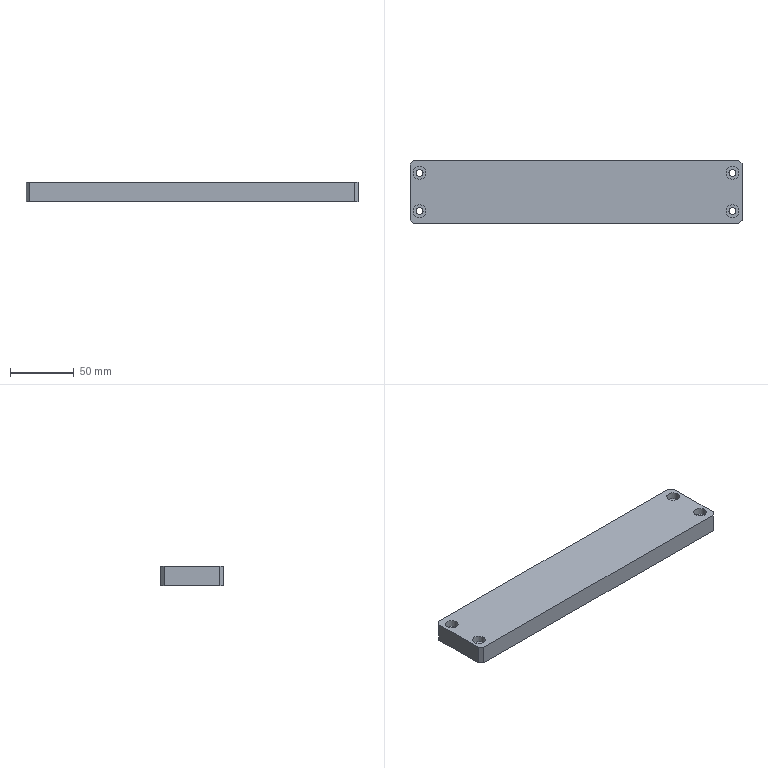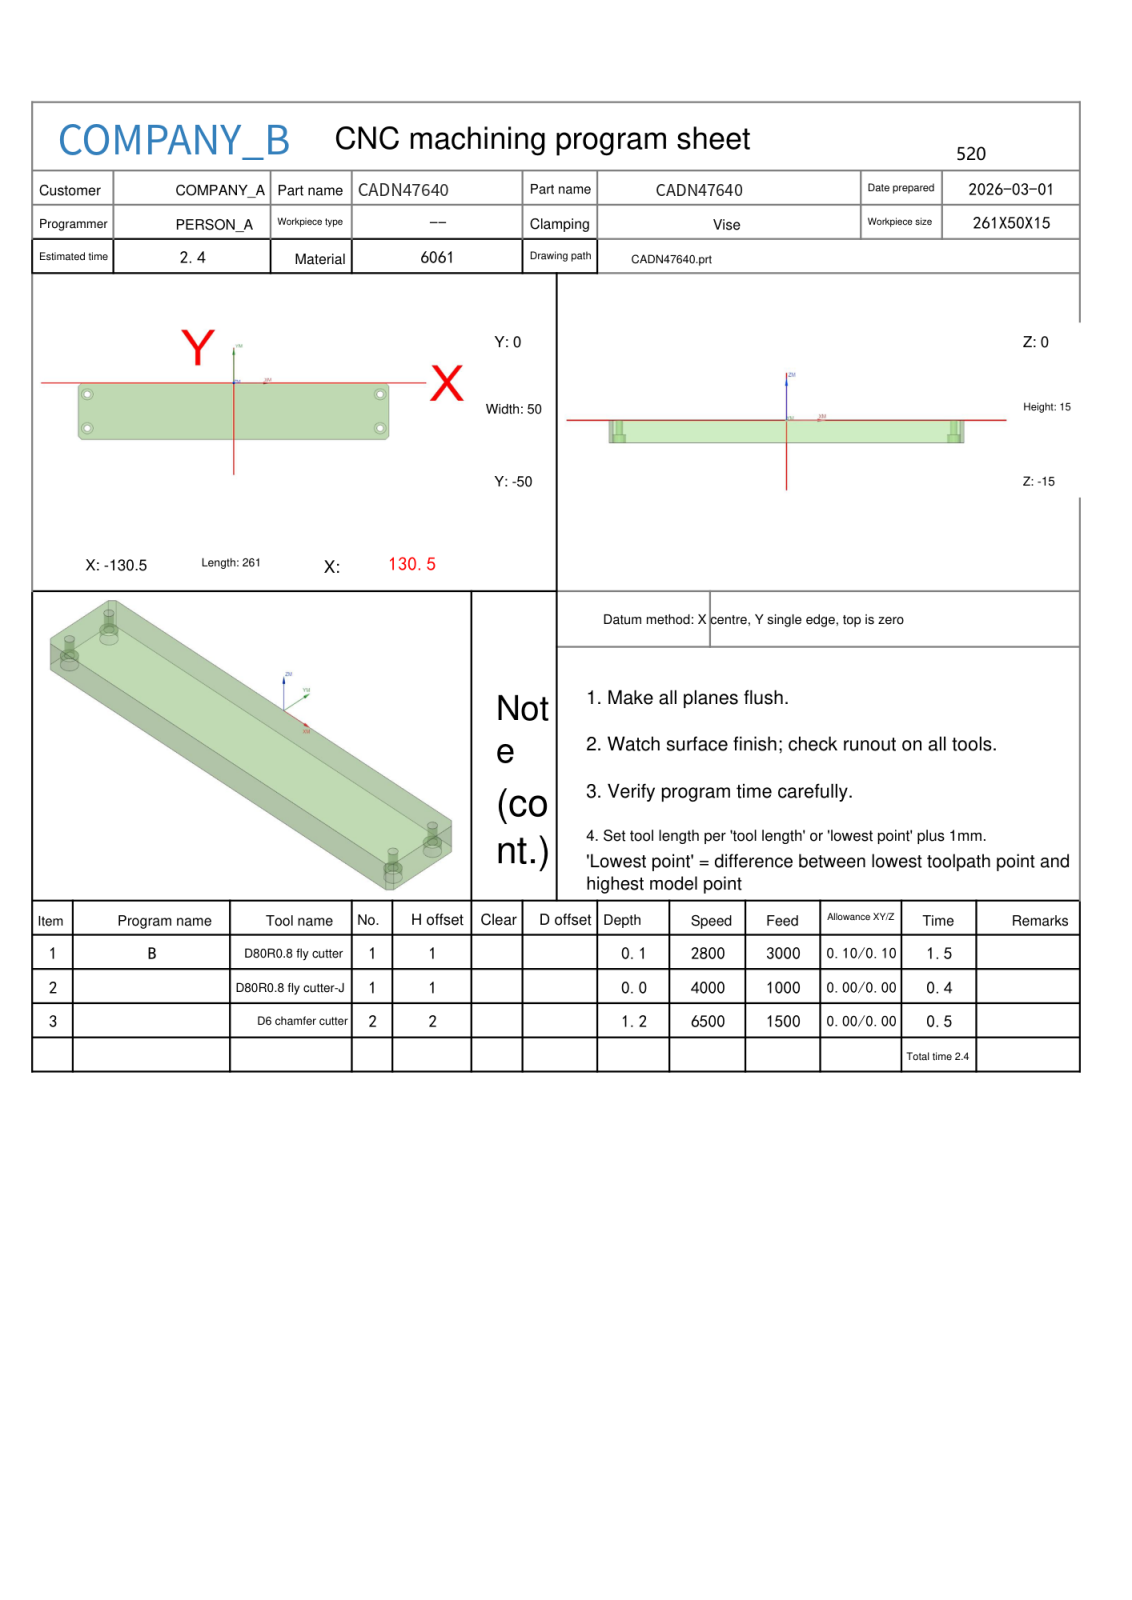NC program | NX | posted by the shop | part box 261 x 50 x 15 mm
Whole program:
%
O0001
(Machine time: 2.86 MIN)
(===Total Tool:2===)
(T1=D80R0.8 fly cutter D=80.  R=0.8  D-  H01 Z=0.    )
(T2=D6 chamfer cutter   D=6.   R=0.   D-  H02 Z=-1.2  )
G80 G90 G17 G49 G40
G91 G28 Z0
M01
N1 T01 M06
(D80R0.8 fly cutter  D=80. R=0.8 H=01 ce=0.10 di=0.10)
G00 G90 G54 X182.597 Y-25. M03 S2800
G43 H01 Z50.
M08
Z6.011
G01 Z4.011 F3000.
X170.597
X-170.597
X-182.597
Z6.011
G00 X182.597
Z5.522
G01 Z3.522
X170.597
X-170.597
X-182.597
Z5.522
G00 X182.597
Z5.033
G01 Z3.033
X170.597
X-170.597
X-182.597
Z5.033
G00 X182.597
Z4.544
G01 Z2.544
X170.597
X-170.597
X-182.597
Z4.544
G00 Z50.
X182.597
Z4.056
G01 Z2.056
X170.597
X-170.597
X-182.597
Z4.056
G00 Z50.
X182.597
Z3.567
G01 Z1.567
X170.597
X-170.597
X-182.597
Z3.567
G00 Z50.
X182.597
Z3.078
G01 Z1.078
X170.597
X-170.597
X-182.597
Z3.078
G00 Z50.
X182.597
Z2.589
G01 Z.589
X170.597
X-170.597
X-182.597
Z2.589
G00 Z50.
X182.597
Z2.1
G01 Z.1
X170.597
X-170.597
X-182.597
Z2.1
G00 Z50.
G91 G28 Z0.0
M05
M09
G91 G28 Z0.0
M01
N2 T01 M06
(D80R0.8 fly cutter-J  D=80. R=0.8 H=01 ce=0.00 di=0.00)
G00 G90 G54 X182.499 Y-25. M03 S4000
G43 H01 Z50.
M08
Z2.
G01 Z0.0 F1000.
X170.499
X-170.499
X-182.499
Z2.
G00 Z50.
G91 G28 Z0.0
M05
M09
G91 G28 Z0.0
M01
N3 T02 M06
(D6 chamfer cutter D=6. R=0. H=02 ce=0.00 di=0.00)
G00 G90 G54 X-.386 Y1.227 M03 S6500
G43 H02 Z50.
M08
Z.172
G01 Z-1.2 F1500.
G03 X-.1 Y1.027 I1.286 J1.532
G01 X-.054 Y.997
X0.0 Y1.
X127.5
X127.759 Y.966
X128. Y.866
X128.207 Y.707
X131.207 Y-2.293
X131.366 Y-2.5
X131.466 Y-2.741
X131.5 Y-3.
Y-47.
X131.466 Y-47.259
X131.366 Y-47.5
X131.207 Y-47.707
X128.207 Y-50.707
X128. Y-50.866
X127.759 Y-50.966
X127.5 Y-51.
X-127.5
X-127.759 Y-50.966
X-128. Y-50.866
X-128.207 Y-50.707
X-131.207 Y-47.707
X-131.366 Y-47.5
X-131.466 Y-47.259
X-131.5 Y-47.
Y-3.
X-131.466 Y-2.741
X-131.366 Y-2.5
X-131.207 Y-2.293
X-128.207 Y.707
X-128. Y.866
X-127.759 Y.966
X-127.5 Y1.
X0.0
X.054 Y.997
X.1 Y1.027
G03 X.386 Y1.227 I-1. J1.732
G01 Z.172
G00 Z10.
X121.435 Y-39.593
Z.27
G01 Z-1.2
G03 X121.266 Y-39.898 I1.658 J-1.118
G01 X121.241 Y-39.946
X121.25 Y-40.
G03 X123. Y-41.75 I1.75 J0.0
X124.75 Y-40. I0.0 J1.75
X123. Y-38.25 I-1.75 J0.0
X121.25 Y-40. I0.0 J-1.75
G01 X121.241 Y-40.054
X121.266 Y-40.102
G03 X121.435 Y-40.407 I1.827 J.813
G01 Z.27
G00 Z10.
Y-9.593
Z.27
G01 Z-1.2
G03 X121.266 Y-9.898 I1.658 J-1.118
G01 X121.241 Y-9.946
X121.25 Y-10.
G03 X123. Y-11.75 I1.75 J0.0
X124.75 Y-10. I0.0 J1.75
X123. Y-8.25 I-1.75 J0.0
X121.25 Y-10. I0.0 J-1.75
G01 X121.241 Y-10.054
X121.266 Y-10.102
G03 X121.435 Y-10.407 I1.827 J.813
G01 Z.27
G00 Z10.
X-124.565 Y-9.593
Z.27
G01 Z-1.2
G03 X-124.734 Y-9.898 I1.658 J-1.118
G01 X-124.759 Y-9.946
X-124.75 Y-10.
G03 X-123. Y-11.75 I1.75 J0.0
X-121.25 Y-10. I0.0 J1.75
X-123. Y-8.25 I-1.75 J0.0
X-124.75 Y-10. I0.0 J-1.75
G01 X-124.759 Y-10.054
X-124.734 Y-10.102
G03 X-124.565 Y-10.407 I1.827 J.813
G01 Z.27
G00 Z10.
Y-39.593
Z.27
G01 Z-1.2
G03 X-124.734 Y-39.898 I1.658 J-1.118
G01 X-124.759 Y-39.946
X-124.75 Y-40.
G03 X-123. Y-41.75 I1.75 J0.0
X-121.25 Y-40. I0.0 J1.75
X-123. Y-38.25 I-1.75 J0.0
X-124.75 Y-40. I0.0 J-1.75
G01 X-124.759 Y-40.054
X-124.734 Y-40.102
G03 X-124.565 Y-40.407 I1.827 J.813
G01 Z.27
G00 Z50.
M05
M09
G91 G28 Z0.0
G91 G28 Y0.0
M30
%